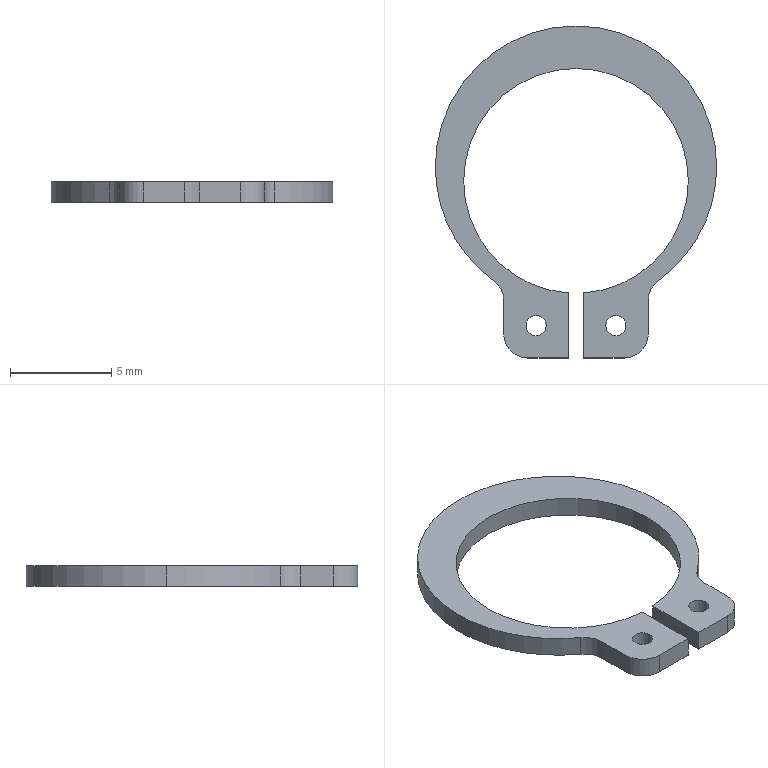Part | NX | features BREP 1 | 1 solid | 22 faces | box 13.9 x 16.4 x 1 mm | volume 70.676 mm3 | cylinder 14 | plane 8 | commonest cylinder face diameters 1 x4 2.38 x4 11.1 x3 13.9 x3
STEP:
#1=CARTESIAN_POINT('',(-2.47,-7.15,0.5));
#2=VERTEX_POINT('',#1);
#3=CARTESIAN_POINT('',(-1.47,-7.15,0.5));
#4=VERTEX_POINT('',#3);
#5=CARTESIAN_POINT('',(-1.97,-7.15,0.5));
#6=DIRECTION('',(0.,0.,1.));
#7=DIRECTION('',(1.,0.,0.));
#8=AXIS2_PLACEMENT_3D('',#5,#6,#7);
#9=CIRCLE('',#8,0.5);
#10=EDGE_CURVE('',#2,#4,#9,.T.);
#11=ORIENTED_EDGE('',*,*,#10,.T.);
#12=CARTESIAN_POINT('',(-1.47,-7.15,-0.5));
#13=VERTEX_POINT('',#12);
#14=CARTESIAN_POINT('',(-1.47,-7.15,0.5));
#15=DIRECTION('',(0.,0.,-1.));
#16=VECTOR('',#15,1000.);
#17=LINE('',#14,#16);
#18=EDGE_CURVE('',#13,#4,#17,.F.);
#19=ORIENTED_EDGE('',*,*,#18,.F.);
#20=CARTESIAN_POINT('',(-2.47,-7.15,-0.5));
#21=VERTEX_POINT('',#20);
#22=CARTESIAN_POINT('',(-1.97,-7.15,-0.5));
#23=DIRECTION('',(0.,0.,1.));
#24=DIRECTION('',(1.,0.,0.));
#25=AXIS2_PLACEMENT_3D('',#22,#23,#24);
#26=CIRCLE('',#25,0.5);
#27=EDGE_CURVE('',#21,#13,#26,.T.);
#28=ORIENTED_EDGE('',*,*,#27,.F.);
#29=CARTESIAN_POINT('',(-2.47,-7.15,0.5));
#30=DIRECTION('',(0.,0.,-1.));
#31=VECTOR('',#30,1000.);
#32=LINE('',#29,#31);
#33=EDGE_CURVE('',#21,#2,#32,.F.);
#34=ORIENTED_EDGE('',*,*,#33,.T.);
#35=EDGE_LOOP('',(#11,#19,#28,#34));
#36=FACE_BOUND('',#35,.T.);
#37=CARTESIAN_POINT('',(-1.97,-7.15,0.5));
#38=DIRECTION('',(0.,0.,-1.));
#39=DIRECTION('',(1.,0.,0.));
#40=AXIS2_PLACEMENT_3D('',#37,#38,#39);
#41=CYLINDRICAL_SURFACE('',#40,0.5);
#42=ADVANCED_FACE('',(#36),#41,.F.);
#43=CARTESIAN_POINT('',(1.47,-7.15,0.5));
#44=VERTEX_POINT('',#43);
#45=CARTESIAN_POINT('',(2.47,-7.15,0.5));
#46=VERTEX_POINT('',#45);
#47=CARTESIAN_POINT('',(1.97,-7.15,0.5));
#48=DIRECTION('',(0.,0.,1.));
#49=DIRECTION('',(1.,0.,0.));
#50=AXIS2_PLACEMENT_3D('',#47,#48,#49);
#51=CIRCLE('',#50,0.5);
#52=EDGE_CURVE('',#44,#46,#51,.T.);
#53=ORIENTED_EDGE('',*,*,#52,.T.);
#54=CARTESIAN_POINT('',(2.47,-7.15,-0.5));
#55=VERTEX_POINT('',#54);
#56=CARTESIAN_POINT('',(2.47,-7.15,0.5));
#57=DIRECTION('',(0.,0.,-1.));
#58=VECTOR('',#57,1000.);
#59=LINE('',#56,#58);
#60=EDGE_CURVE('',#55,#46,#59,.F.);
#61=ORIENTED_EDGE('',*,*,#60,.F.);
#62=CARTESIAN_POINT('',(1.47,-7.15,-0.5));
#63=VERTEX_POINT('',#62);
#64=CARTESIAN_POINT('',(1.97,-7.15,-0.5));
#65=DIRECTION('',(0.,0.,1.));
#66=DIRECTION('',(1.,0.,0.));
#67=AXIS2_PLACEMENT_3D('',#64,#65,#66);
#68=CIRCLE('',#67,0.5);
#69=EDGE_CURVE('',#63,#55,#68,.T.);
#70=ORIENTED_EDGE('',*,*,#69,.F.);
#71=CARTESIAN_POINT('',(1.47,-7.15,0.5));
#72=DIRECTION('',(0.,0.,-1.));
#73=VECTOR('',#72,1000.);
#74=LINE('',#71,#73);
#75=EDGE_CURVE('',#63,#44,#74,.F.);
#76=ORIENTED_EDGE('',*,*,#75,.T.);
#77=EDGE_LOOP('',(#53,#61,#70,#76));
#78=FACE_BOUND('',#77,.T.);
#79=CARTESIAN_POINT('',(1.97,-7.15,0.5));
#80=DIRECTION('',(0.,0.,-1.));
#81=DIRECTION('',(1.,0.,0.));
#82=AXIS2_PLACEMENT_3D('',#79,#80,#81);
#83=CYLINDRICAL_SURFACE('',#82,0.5);
#84=ADVANCED_FACE('',(#78),#83,.F.);
#85=CARTESIAN_POINT('',(5.55,0.,0.5));
#86=VERTEX_POINT('',#85);
#87=CARTESIAN_POINT('',(0.37,-5.538,0.5));
#88=VERTEX_POINT('',#87);
#89=CARTESIAN_POINT('',(0.,0.,0.5));
#90=DIRECTION('',(0.,0.,-1.));
#91=DIRECTION('',(-1.,0.,0.));
#92=AXIS2_PLACEMENT_3D('',#89,#90,#91);
#93=CIRCLE('',#92,5.55);
#94=EDGE_CURVE('',#86,#88,#93,.T.);
#95=ORIENTED_EDGE('',*,*,#94,.F.);
#96=CARTESIAN_POINT('',(5.55,0.,-0.5));
#97=VERTEX_POINT('',#96);
#98=CARTESIAN_POINT('',(5.55,0.,0.5));
#99=DIRECTION('',(0.,0.,-1.));
#100=VECTOR('',#99,1000.);
#101=LINE('',#98,#100);
#102=EDGE_CURVE('',#86,#97,#101,.T.);
#103=ORIENTED_EDGE('',*,*,#102,.T.);
#104=CARTESIAN_POINT('',(0.37,-5.538,-0.5));
#105=VERTEX_POINT('',#104);
#106=CARTESIAN_POINT('',(0.,0.,-0.5));
#107=DIRECTION('',(0.,0.,-1.));
#108=DIRECTION('',(-1.,0.,0.));
#109=AXIS2_PLACEMENT_3D('',#106,#107,#108);
#110=CIRCLE('',#109,5.55);
#111=EDGE_CURVE('',#97,#105,#110,.T.);
#112=ORIENTED_EDGE('',*,*,#111,.T.);
#113=CARTESIAN_POINT('',(0.37,-5.538,0.5));
#114=DIRECTION('',(0.,0.,-1.));
#115=VECTOR('',#114,1000.);
#116=LINE('',#113,#115);
#117=EDGE_CURVE('',#88,#105,#116,.T.);
#118=ORIENTED_EDGE('',*,*,#117,.F.);
#119=EDGE_LOOP('',(#95,#103,#112,#118));
#120=FACE_BOUND('',#119,.T.);
#121=CARTESIAN_POINT('',(0.,0.,0.5));
#122=DIRECTION('',(0.,0.,-1.));
#123=DIRECTION('',(1.,0.,0.));
#124=AXIS2_PLACEMENT_3D('',#121,#122,#123);
#125=CYLINDRICAL_SURFACE('',#124,5.55);
#126=ADVANCED_FACE('',(#120),#125,.F.);
#127=ORIENTED_EDGE('',*,*,#102,.F.);
#128=CARTESIAN_POINT('',(-5.55,0.,0.5));
#129=VERTEX_POINT('',#128);
#130=CARTESIAN_POINT('',(0.,0.,0.5));
#131=DIRECTION('',(0.,0.,-1.));
#132=DIRECTION('',(-1.,0.,0.));
#133=AXIS2_PLACEMENT_3D('',#130,#131,#132);
#134=CIRCLE('',#133,5.55);
#135=EDGE_CURVE('',#129,#86,#134,.T.);
#136=ORIENTED_EDGE('',*,*,#135,.F.);
#137=CARTESIAN_POINT('',(-5.55,0.,-0.5));
#138=VERTEX_POINT('',#137);
#139=CARTESIAN_POINT('',(-5.55,0.,0.5));
#140=DIRECTION('',(0.,0.,-1.));
#141=VECTOR('',#140,1000.);
#142=LINE('',#139,#141);
#143=EDGE_CURVE('',#129,#138,#142,.T.);
#144=ORIENTED_EDGE('',*,*,#143,.T.);
#145=CARTESIAN_POINT('',(0.,0.,-0.5));
#146=DIRECTION('',(0.,0.,-1.));
#147=DIRECTION('',(-1.,0.,0.));
#148=AXIS2_PLACEMENT_3D('',#145,#146,#147);
#149=CIRCLE('',#148,5.55);
#150=EDGE_CURVE('',#138,#97,#149,.T.);
#151=ORIENTED_EDGE('',*,*,#150,.T.);
#152=EDGE_LOOP('',(#127,#136,#144,#151));
#153=FACE_BOUND('',#152,.T.);
#154=CARTESIAN_POINT('',(0.,0.,0.5));
#155=DIRECTION('',(0.,0.,-1.));
#156=DIRECTION('',(1.,0.,0.));
#157=AXIS2_PLACEMENT_3D('',#154,#155,#156);
#158=CYLINDRICAL_SURFACE('',#157,5.55);
#159=ADVANCED_FACE('',(#153),#158,.F.);
#160=CARTESIAN_POINT('',(6.95,0.7,0.5));
#161=VERTEX_POINT('',#160);
#162=CARTESIAN_POINT('',(-6.95,0.7,0.5));
#163=VERTEX_POINT('',#162);
#164=CARTESIAN_POINT('',(0.,0.7,0.5));
#165=DIRECTION('',(0.,0.,1.));
#166=DIRECTION('',(1.,0.,0.));
#167=AXIS2_PLACEMENT_3D('',#164,#165,#166);
#168=CIRCLE('',#167,6.95);
#169=EDGE_CURVE('',#161,#163,#168,.T.);
#170=ORIENTED_EDGE('',*,*,#169,.F.);
#171=CARTESIAN_POINT('',(6.95,0.7,-0.5));
#172=VERTEX_POINT('',#171);
#173=CARTESIAN_POINT('',(6.95,0.7,0.5));
#174=DIRECTION('',(0.,0.,-1.));
#175=VECTOR('',#174,1000.);
#176=LINE('',#173,#175);
#177=EDGE_CURVE('',#161,#172,#176,.T.);
#178=ORIENTED_EDGE('',*,*,#177,.T.);
#179=CARTESIAN_POINT('',(-6.95,0.7,-0.5));
#180=VERTEX_POINT('',#179);
#181=CARTESIAN_POINT('',(0.,0.7,-0.5));
#182=DIRECTION('',(0.,0.,1.));
#183=DIRECTION('',(1.,0.,0.));
#184=AXIS2_PLACEMENT_3D('',#181,#182,#183);
#185=CIRCLE('',#184,6.95);
#186=EDGE_CURVE('',#172,#180,#185,.T.);
#187=ORIENTED_EDGE('',*,*,#186,.T.);
#188=CARTESIAN_POINT('',(-6.95,0.7,0.5));
#189=DIRECTION('',(0.,0.,-1.));
#190=VECTOR('',#189,1000.);
#191=LINE('',#188,#190);
#192=EDGE_CURVE('',#163,#180,#191,.T.);
#193=ORIENTED_EDGE('',*,*,#192,.F.);
#194=EDGE_LOOP('',(#170,#178,#187,#193));
#195=FACE_BOUND('',#194,.T.);
#196=CARTESIAN_POINT('',(0.,0.7,0.5));
#197=DIRECTION('',(0.,0.,-1.));
#198=DIRECTION('',(1.,0.,0.));
#199=AXIS2_PLACEMENT_3D('',#196,#197,#198);
#200=CYLINDRICAL_SURFACE('',#199,6.95);
#201=ADVANCED_FACE('',(#195),#200,.T.);
#202=CARTESIAN_POINT('',(-4.064,-4.938,0.5));
#203=VERTEX_POINT('',#202);
#204=CARTESIAN_POINT('',(0.,0.7,0.5));
#205=DIRECTION('',(0.,0.,1.));
#206=DIRECTION('',(1.,0.,0.));
#207=AXIS2_PLACEMENT_3D('',#204,#205,#206);
#208=CIRCLE('',#207,6.95);
#209=EDGE_CURVE('',#163,#203,#208,.T.);
#210=ORIENTED_EDGE('',*,*,#209,.F.);
#211=ORIENTED_EDGE('',*,*,#192,.T.);
#212=CARTESIAN_POINT('',(-4.064,-4.938,-0.5));
#213=VERTEX_POINT('',#212);
#214=CARTESIAN_POINT('',(0.,0.7,-0.5));
#215=DIRECTION('',(0.,0.,1.));
#216=DIRECTION('',(1.,0.,0.));
#217=AXIS2_PLACEMENT_3D('',#214,#215,#216);
#218=CIRCLE('',#217,6.95);
#219=EDGE_CURVE('',#180,#213,#218,.T.);
#220=ORIENTED_EDGE('',*,*,#219,.T.);
#221=CARTESIAN_POINT('',(-4.064,-4.938,0.5));
#222=DIRECTION('',(0.,0.,-1.));
#223=VECTOR('',#222,1000.);
#224=LINE('',#221,#223);
#225=EDGE_CURVE('',#203,#213,#224,.T.);
#226=ORIENTED_EDGE('',*,*,#225,.F.);
#227=EDGE_LOOP('',(#210,#211,#220,#226));
#228=FACE_BOUND('',#227,.T.);
#229=CARTESIAN_POINT('',(0.,0.7,0.5));
#230=DIRECTION('',(0.,0.,-1.));
#231=DIRECTION('',(1.,0.,0.));
#232=AXIS2_PLACEMENT_3D('',#229,#230,#231);
#233=CYLINDRICAL_SURFACE('',#232,6.95);
#234=ADVANCED_FACE('',(#228),#233,.T.);
#235=CARTESIAN_POINT('',(3.57,-5.903,0.5));
#236=VERTEX_POINT('',#235);
#237=CARTESIAN_POINT('',(4.064,-4.938,0.5));
#238=VERTEX_POINT('',#237);
#239=CARTESIAN_POINT('',(4.76,-5.903,0.5));
#240=DIRECTION('',(0.,0.,-1.));
#241=DIRECTION('',(-1.,0.,0.));
#242=AXIS2_PLACEMENT_3D('',#239,#240,#241);
#243=CIRCLE('',#242,1.19);
#244=EDGE_CURVE('',#236,#238,#243,.T.);
#245=ORIENTED_EDGE('',*,*,#244,.T.);
#246=CARTESIAN_POINT('',(0.,0.7,0.5));
#247=DIRECTION('',(0.,0.,1.));
#248=DIRECTION('',(1.,0.,0.));
#249=AXIS2_PLACEMENT_3D('',#246,#247,#248);
#250=CIRCLE('',#249,6.95);
#251=EDGE_CURVE('',#238,#161,#250,.T.);
#252=ORIENTED_EDGE('',*,*,#251,.T.);
#253=ORIENTED_EDGE('',*,*,#169,.T.);
#254=ORIENTED_EDGE('',*,*,#209,.T.);
#255=CARTESIAN_POINT('',(-3.57,-5.903,0.5));
#256=VERTEX_POINT('',#255);
#257=CARTESIAN_POINT('',(-4.76,-5.903,0.5));
#258=DIRECTION('',(0.,0.,-1.));
#259=DIRECTION('',(-1.,0.,0.));
#260=AXIS2_PLACEMENT_3D('',#257,#258,#259);
#261=CIRCLE('',#260,1.19);
#262=EDGE_CURVE('',#203,#256,#261,.T.);
#263=ORIENTED_EDGE('',*,*,#262,.T.);
#264=CARTESIAN_POINT('',(-3.57,-7.56,0.5));
#265=VERTEX_POINT('',#264);
#266=CARTESIAN_POINT('',(-3.57,-5.903,0.5));
#267=DIRECTION('',(0.,-1.,0.));
#268=VECTOR('',#267,1000.);
#269=LINE('',#266,#268);
#270=EDGE_CURVE('',#256,#265,#269,.T.);
#271=ORIENTED_EDGE('',*,*,#270,.T.);
#272=CARTESIAN_POINT('',(-2.38,-8.75,0.5));
#273=VERTEX_POINT('',#272);
#274=CARTESIAN_POINT('',(-2.38,-7.56,0.5));
#275=DIRECTION('',(0.,0.,1.));
#276=DIRECTION('',(1.,0.,0.));
#277=AXIS2_PLACEMENT_3D('',#274,#275,#276);
#278=CIRCLE('',#277,1.19);
#279=EDGE_CURVE('',#265,#273,#278,.T.);
#280=ORIENTED_EDGE('',*,*,#279,.T.);
#281=CARTESIAN_POINT('',(-0.37,-8.75,0.5));
#282=VERTEX_POINT('',#281);
#283=CARTESIAN_POINT('',(-2.38,-8.75,0.5));
#284=DIRECTION('',(1.,0.,0.));
#285=VECTOR('',#284,1000.);
#286=LINE('',#283,#285);
#287=EDGE_CURVE('',#273,#282,#286,.T.);
#288=ORIENTED_EDGE('',*,*,#287,.T.);
#289=CARTESIAN_POINT('',(-0.37,-5.538,0.5));
#290=VERTEX_POINT('',#289);
#291=CARTESIAN_POINT('',(-0.37,-8.75,0.5));
#292=DIRECTION('',(0.,1.,0.));
#293=VECTOR('',#292,1000.);
#294=LINE('',#291,#293);
#295=EDGE_CURVE('',#282,#290,#294,.T.);
#296=ORIENTED_EDGE('',*,*,#295,.T.);
#297=CARTESIAN_POINT('',(0.,0.,0.5));
#298=DIRECTION('',(0.,0.,-1.));
#299=DIRECTION('',(-1.,0.,0.));
#300=AXIS2_PLACEMENT_3D('',#297,#298,#299);
#301=CIRCLE('',#300,5.55);
#302=EDGE_CURVE('',#290,#129,#301,.T.);
#303=ORIENTED_EDGE('',*,*,#302,.T.);
#304=ORIENTED_EDGE('',*,*,#135,.T.);
#305=ORIENTED_EDGE('',*,*,#94,.T.);
#306=CARTESIAN_POINT('',(0.37,-8.75,0.5));
#307=VERTEX_POINT('',#306);
#308=CARTESIAN_POINT('',(0.37,-5.538,0.5));
#309=DIRECTION('',(0.,-1.,0.));
#310=VECTOR('',#309,1000.);
#311=LINE('',#308,#310);
#312=EDGE_CURVE('',#88,#307,#311,.T.);
#313=ORIENTED_EDGE('',*,*,#312,.T.);
#314=CARTESIAN_POINT('',(2.38,-8.75,0.5));
#315=VERTEX_POINT('',#314);
#316=CARTESIAN_POINT('',(0.37,-8.75,0.5));
#317=DIRECTION('',(1.,0.,0.));
#318=VECTOR('',#317,1000.);
#319=LINE('',#316,#318);
#320=EDGE_CURVE('',#307,#315,#319,.T.);
#321=ORIENTED_EDGE('',*,*,#320,.T.);
#322=CARTESIAN_POINT('',(3.57,-7.56,0.5));
#323=VERTEX_POINT('',#322);
#324=CARTESIAN_POINT('',(2.38,-7.56,0.5));
#325=DIRECTION('',(0.,0.,1.));
#326=DIRECTION('',(1.,0.,0.));
#327=AXIS2_PLACEMENT_3D('',#324,#325,#326);
#328=CIRCLE('',#327,1.19);
#329=EDGE_CURVE('',#315,#323,#328,.T.);
#330=ORIENTED_EDGE('',*,*,#329,.T.);
#331=CARTESIAN_POINT('',(3.57,-7.56,0.5));
#332=DIRECTION('',(0.,1.,0.));
#333=VECTOR('',#332,1000.);
#334=LINE('',#331,#333);
#335=EDGE_CURVE('',#323,#236,#334,.T.);
#336=ORIENTED_EDGE('',*,*,#335,.T.);
#337=EDGE_LOOP('',(#245,#252,#253,#254,#263,#271,#280,#288,#296,#303,#304,#305,#313,#321,#330,#336));
#338=FACE_BOUND('',#337,.T.);
#339=ORIENTED_EDGE('',*,*,#52,.F.);
#340=CARTESIAN_POINT('',(1.97,-7.15,0.5));
#341=DIRECTION('',(0.,0.,1.));
#342=DIRECTION('',(1.,0.,0.));
#343=AXIS2_PLACEMENT_3D('',#340,#341,#342);
#344=CIRCLE('',#343,0.5);
#345=EDGE_CURVE('',#46,#44,#344,.T.);
#346=ORIENTED_EDGE('',*,*,#345,.F.);
#347=EDGE_LOOP('',(#339,#346));
#348=FACE_BOUND('',#347,.T.);
#349=ORIENTED_EDGE('',*,*,#10,.F.);
#350=CARTESIAN_POINT('',(-1.97,-7.15,0.5));
#351=DIRECTION('',(0.,0.,1.));
#352=DIRECTION('',(1.,0.,0.));
#353=AXIS2_PLACEMENT_3D('',#350,#351,#352);
#354=CIRCLE('',#353,0.5);
#355=EDGE_CURVE('',#4,#2,#354,.T.);
#356=ORIENTED_EDGE('',*,*,#355,.F.);
#357=EDGE_LOOP('',(#349,#356));
#358=FACE_BOUND('',#357,.T.);
#359=CARTESIAN_POINT('',(4.76,-5.903,0.5));
#360=DIRECTION('',(0.,0.,-1.));
#361=DIRECTION('',(1.,0.,0.));
#362=AXIS2_PLACEMENT_3D('',#359,#360,#361);
#363=PLANE('',#362);
#364=ADVANCED_FACE('',(#338,#348,#358),#363,.F.);
#365=CARTESIAN_POINT('',(3.57,-5.903,-0.5));
#366=VERTEX_POINT('',#365);
#367=CARTESIAN_POINT('',(3.57,-5.903,0.5));
#368=DIRECTION('',(0.,0.,-1.));
#369=VECTOR('',#368,1000.);
#370=LINE('',#367,#369);
#371=EDGE_CURVE('',#236,#366,#370,.T.);
#372=ORIENTED_EDGE('',*,*,#371,.T.);
#373=CARTESIAN_POINT('',(4.064,-4.938,-0.5));
#374=VERTEX_POINT('',#373);
#375=CARTESIAN_POINT('',(4.76,-5.903,-0.5));
#376=DIRECTION('',(0.,0.,-1.));
#377=DIRECTION('',(-1.,0.,0.));
#378=AXIS2_PLACEMENT_3D('',#375,#376,#377);
#379=CIRCLE('',#378,1.19);
#380=EDGE_CURVE('',#366,#374,#379,.T.);
#381=ORIENTED_EDGE('',*,*,#380,.T.);
#382=CARTESIAN_POINT('',(4.064,-4.938,0.5));
#383=DIRECTION('',(0.,0.,-1.));
#384=VECTOR('',#383,1000.);
#385=LINE('',#382,#384);
#386=EDGE_CURVE('',#238,#374,#385,.T.);
#387=ORIENTED_EDGE('',*,*,#386,.F.);
#388=ORIENTED_EDGE('',*,*,#244,.F.);
#389=EDGE_LOOP('',(#372,#381,#387,#388));
#390=FACE_BOUND('',#389,.T.);
#391=CARTESIAN_POINT('',(4.76,-5.903,0.5));
#392=DIRECTION('',(0.,0.,-1.));
#393=DIRECTION('',(1.,0.,0.));
#394=AXIS2_PLACEMENT_3D('',#391,#392,#393);
#395=CYLINDRICAL_SURFACE('',#394,1.19);
#396=ADVANCED_FACE('',(#390),#395,.F.);
#397=ORIENTED_EDGE('',*,*,#177,.F.);
#398=ORIENTED_EDGE('',*,*,#251,.F.);
#399=ORIENTED_EDGE('',*,*,#386,.T.);
#400=CARTESIAN_POINT('',(0.,0.7,-0.5));
#401=DIRECTION('',(0.,0.,1.));
#402=DIRECTION('',(1.,0.,0.));
#403=AXIS2_PLACEMENT_3D('',#400,#401,#402);
#404=CIRCLE('',#403,6.95);
#405=EDGE_CURVE('',#374,#172,#404,.T.);
#406=ORIENTED_EDGE('',*,*,#405,.T.);
#407=EDGE_LOOP('',(#397,#398,#399,#406));
#408=FACE_BOUND('',#407,.T.);
#409=CARTESIAN_POINT('',(0.,0.7,0.5));
#410=DIRECTION('',(0.,0.,-1.));
#411=DIRECTION('',(1.,0.,0.));
#412=AXIS2_PLACEMENT_3D('',#409,#410,#411);
#413=CYLINDRICAL_SURFACE('',#412,6.95);
#414=ADVANCED_FACE('',(#408),#413,.T.);
#415=ORIENTED_EDGE('',*,*,#225,.T.);
#416=CARTESIAN_POINT('',(-3.57,-5.903,-0.5));
#417=VERTEX_POINT('',#416);
#418=CARTESIAN_POINT('',(-4.76,-5.903,-0.5));
#419=DIRECTION('',(0.,0.,-1.));
#420=DIRECTION('',(-1.,0.,0.));
#421=AXIS2_PLACEMENT_3D('',#418,#419,#420);
#422=CIRCLE('',#421,1.19);
#423=EDGE_CURVE('',#213,#417,#422,.T.);
#424=ORIENTED_EDGE('',*,*,#423,.T.);
#425=CARTESIAN_POINT('',(-3.57,-5.903,0.5));
#426=DIRECTION('',(0.,0.,-1.));
#427=VECTOR('',#426,1000.);
#428=LINE('',#425,#427);
#429=EDGE_CURVE('',#256,#417,#428,.T.);
#430=ORIENTED_EDGE('',*,*,#429,.F.);
#431=ORIENTED_EDGE('',*,*,#262,.F.);
#432=EDGE_LOOP('',(#415,#424,#430,#431));
#433=FACE_BOUND('',#432,.T.);
#434=CARTESIAN_POINT('',(-4.76,-5.903,0.5));
#435=DIRECTION('',(0.,0.,-1.));
#436=DIRECTION('',(1.,0.,0.));
#437=AXIS2_PLACEMENT_3D('',#434,#435,#436);
#438=CYLINDRICAL_SURFACE('',#437,1.19);
#439=ADVANCED_FACE('',(#433),#438,.F.);
#440=ORIENTED_EDGE('',*,*,#429,.T.);
#441=CARTESIAN_POINT('',(-3.57,-7.56,-0.5));
#442=VERTEX_POINT('',#441);
#443=CARTESIAN_POINT('',(-3.57,-5.903,-0.5));
#444=DIRECTION('',(0.,-1.,0.));
#445=VECTOR('',#444,1000.);
#446=LINE('',#443,#445);
#447=EDGE_CURVE('',#417,#442,#446,.T.);
#448=ORIENTED_EDGE('',*,*,#447,.T.);
#449=CARTESIAN_POINT('',(-3.57,-7.56,0.5));
#450=DIRECTION('',(0.,0.,-1.));
#451=VECTOR('',#450,1000.);
#452=LINE('',#449,#451);
#453=EDGE_CURVE('',#265,#442,#452,.T.);
#454=ORIENTED_EDGE('',*,*,#453,.F.);
#455=ORIENTED_EDGE('',*,*,#270,.F.);
#456=EDGE_LOOP('',(#440,#448,#454,#455));
#457=FACE_BOUND('',#456,.T.);
#458=CARTESIAN_POINT('',(-3.57,-5.903,0.5));
#459=DIRECTION('',(1.,0.,0.));
#460=DIRECTION('',(0.,0.,1.));
#461=AXIS2_PLACEMENT_3D('',#458,#459,#460);
#462=PLANE('',#461);
#463=ADVANCED_FACE('',(#457),#462,.F.);
#464=ORIENTED_EDGE('',*,*,#453,.T.);
#465=CARTESIAN_POINT('',(-2.38,-8.75,-0.5));
#466=VERTEX_POINT('',#465);
#467=CARTESIAN_POINT('',(-2.38,-7.56,-0.5));
#468=DIRECTION('',(0.,0.,1.));
#469=DIRECTION('',(1.,0.,0.));
#470=AXIS2_PLACEMENT_3D('',#467,#468,#469);
#471=CIRCLE('',#470,1.19);
#472=EDGE_CURVE('',#442,#466,#471,.T.);
#473=ORIENTED_EDGE('',*,*,#472,.T.);
#474=CARTESIAN_POINT('',(-2.38,-8.75,0.5));
#475=DIRECTION('',(0.,0.,-1.));
#476=VECTOR('',#475,1000.);
#477=LINE('',#474,#476);
#478=EDGE_CURVE('',#273,#466,#477,.T.);
#479=ORIENTED_EDGE('',*,*,#478,.F.);
#480=ORIENTED_EDGE('',*,*,#279,.F.);
#481=EDGE_LOOP('',(#464,#473,#479,#480));
#482=FACE_BOUND('',#481,.T.);
#483=CARTESIAN_POINT('',(-2.38,-7.56,0.5));
#484=DIRECTION('',(0.,0.,-1.));
#485=DIRECTION('',(1.,0.,0.));
#486=AXIS2_PLACEMENT_3D('',#483,#484,#485);
#487=CYLINDRICAL_SURFACE('',#486,1.19);
#488=ADVANCED_FACE('',(#482),#487,.T.);
#489=ORIENTED_EDGE('',*,*,#478,.T.);
#490=CARTESIAN_POINT('',(-0.37,-8.75,-0.5));
#491=VERTEX_POINT('',#490);
#492=CARTESIAN_POINT('',(-2.38,-8.75,-0.5));
#493=DIRECTION('',(1.,0.,0.));
#494=VECTOR('',#493,1000.);
#495=LINE('',#492,#494);
#496=EDGE_CURVE('',#466,#491,#495,.T.);
#497=ORIENTED_EDGE('',*,*,#496,.T.);
#498=CARTESIAN_POINT('',(-0.37,-8.75,0.5));
#499=DIRECTION('',(0.,0.,-1.));
#500=VECTOR('',#499,1000.);
#501=LINE('',#498,#500);
#502=EDGE_CURVE('',#282,#491,#501,.T.);
#503=ORIENTED_EDGE('',*,*,#502,.F.);
#504=ORIENTED_EDGE('',*,*,#287,.F.);
#505=EDGE_LOOP('',(#489,#497,#503,#504));
#506=FACE_BOUND('',#505,.T.);
#507=CARTESIAN_POINT('',(-2.38,-8.75,0.5));
#508=DIRECTION('',(0.,1.,0.));
#509=DIRECTION('',(0.,0.,-1.));
#510=AXIS2_PLACEMENT_3D('',#507,#508,#509);
#511=PLANE('',#510);
#512=ADVANCED_FACE('',(#506),#511,.F.);
#513=ORIENTED_EDGE('',*,*,#502,.T.);
#514=CARTESIAN_POINT('',(-0.37,-5.538,-0.5));
#515=VERTEX_POINT('',#514);
#516=CARTESIAN_POINT('',(-0.37,-8.75,-0.5));
#517=DIRECTION('',(0.,1.,0.));
#518=VECTOR('',#517,1000.);
#519=LINE('',#516,#518);
#520=EDGE_CURVE('',#491,#515,#519,.T.);
#521=ORIENTED_EDGE('',*,*,#520,.T.);
#522=CARTESIAN_POINT('',(-0.37,-5.538,0.5));
#523=DIRECTION('',(0.,0.,-1.));
#524=VECTOR('',#523,1000.);
#525=LINE('',#522,#524);
#526=EDGE_CURVE('',#290,#515,#525,.T.);
#527=ORIENTED_EDGE('',*,*,#526,.F.);
#528=ORIENTED_EDGE('',*,*,#295,.F.);
#529=EDGE_LOOP('',(#513,#521,#527,#528));
#530=FACE_BOUND('',#529,.T.);
#531=CARTESIAN_POINT('',(-0.37,-8.75,0.5));
#532=DIRECTION('',(-1.,0.,0.));
#533=DIRECTION('',(0.,0.,-1.));
#534=AXIS2_PLACEMENT_3D('',#531,#532,#533);
#535=PLANE('',#534);
#536=ADVANCED_FACE('',(#530),#535,.F.);
#537=ORIENTED_EDGE('',*,*,#143,.F.);
#538=ORIENTED_EDGE('',*,*,#302,.F.);
#539=ORIENTED_EDGE('',*,*,#526,.T.);
#540=CARTESIAN_POINT('',(0.,0.,-0.5));
#541=DIRECTION('',(0.,0.,-1.));
#542=DIRECTION('',(-1.,0.,0.));
#543=AXIS2_PLACEMENT_3D('',#540,#541,#542);
#544=CIRCLE('',#543,5.55);
#545=EDGE_CURVE('',#515,#138,#544,.T.);
#546=ORIENTED_EDGE('',*,*,#545,.T.);
#547=EDGE_LOOP('',(#537,#538,#539,#546));
#548=FACE_BOUND('',#547,.T.);
#549=CARTESIAN_POINT('',(0.,0.,0.5));
#550=DIRECTION('',(0.,0.,-1.));
#551=DIRECTION('',(1.,0.,0.));
#552=AXIS2_PLACEMENT_3D('',#549,#550,#551);
#553=CYLINDRICAL_SURFACE('',#552,5.55);
#554=ADVANCED_FACE('',(#548),#553,.F.);
#555=ORIENTED_EDGE('',*,*,#117,.T.);
#556=CARTESIAN_POINT('',(0.37,-8.75,-0.5));
#557=VERTEX_POINT('',#556);
#558=CARTESIAN_POINT('',(0.37,-5.538,-0.5));
#559=DIRECTION('',(0.,-1.,0.));
#560=VECTOR('',#559,1000.);
#561=LINE('',#558,#560);
#562=EDGE_CURVE('',#105,#557,#561,.T.);
#563=ORIENTED_EDGE('',*,*,#562,.T.);
#564=CARTESIAN_POINT('',(0.37,-8.75,0.5));
#565=DIRECTION('',(0.,0.,-1.));
#566=VECTOR('',#565,1000.);
#567=LINE('',#564,#566);
#568=EDGE_CURVE('',#307,#557,#567,.T.);
#569=ORIENTED_EDGE('',*,*,#568,.F.);
#570=ORIENTED_EDGE('',*,*,#312,.F.);
#571=EDGE_LOOP('',(#555,#563,#569,#570));
#572=FACE_BOUND('',#571,.T.);
#573=CARTESIAN_POINT('',(0.37,-5.538,0.5));
#574=DIRECTION('',(1.,0.,0.));
#575=DIRECTION('',(0.,0.,1.));
#576=AXIS2_PLACEMENT_3D('',#573,#574,#575);
#577=PLANE('',#576);
#578=ADVANCED_FACE('',(#572),#577,.F.);
#579=ORIENTED_EDGE('',*,*,#568,.T.);
#580=CARTESIAN_POINT('',(2.38,-8.75,-0.5));
#581=VERTEX_POINT('',#580);
#582=CARTESIAN_POINT('',(0.37,-8.75,-0.5));
#583=DIRECTION('',(1.,0.,0.));
#584=VECTOR('',#583,1000.);
#585=LINE('',#582,#584);
#586=EDGE_CURVE('',#557,#581,#585,.T.);
#587=ORIENTED_EDGE('',*,*,#586,.T.);
#588=CARTESIAN_POINT('',(2.38,-8.75,0.5));
#589=DIRECTION('',(0.,0.,-1.));
#590=VECTOR('',#589,1000.);
#591=LINE('',#588,#590);
#592=EDGE_CURVE('',#315,#581,#591,.T.);
#593=ORIENTED_EDGE('',*,*,#592,.F.);
#594=ORIENTED_EDGE('',*,*,#320,.F.);
#595=EDGE_LOOP('',(#579,#587,#593,#594));
#596=FACE_BOUND('',#595,.T.);
#597=CARTESIAN_POINT('',(0.37,-8.75,0.5));
#598=DIRECTION('',(0.,1.,0.));
#599=DIRECTION('',(0.,0.,-1.));
#600=AXIS2_PLACEMENT_3D('',#597,#598,#599);
#601=PLANE('',#600);
#602=ADVANCED_FACE('',(#596),#601,.F.);
#603=ORIENTED_EDGE('',*,*,#592,.T.);
#604=CARTESIAN_POINT('',(3.57,-7.56,-0.5));
#605=VERTEX_POINT('',#604);
#606=CARTESIAN_POINT('',(2.38,-7.56,-0.5));
#607=DIRECTION('',(0.,0.,1.));
#608=DIRECTION('',(1.,0.,0.));
#609=AXIS2_PLACEMENT_3D('',#606,#607,#608);
#610=CIRCLE('',#609,1.19);
#611=EDGE_CURVE('',#581,#605,#610,.T.);
#612=ORIENTED_EDGE('',*,*,#611,.T.);
#613=CARTESIAN_POINT('',(3.57,-7.56,0.5));
#614=DIRECTION('',(0.,0.,-1.));
#615=VECTOR('',#614,1000.);
#616=LINE('',#613,#615);
#617=EDGE_CURVE('',#323,#605,#616,.T.);
#618=ORIENTED_EDGE('',*,*,#617,.F.);
#619=ORIENTED_EDGE('',*,*,#329,.F.);
#620=EDGE_LOOP('',(#603,#612,#618,#619));
#621=FACE_BOUND('',#620,.T.);
#622=CARTESIAN_POINT('',(2.38,-7.56,0.5));
#623=DIRECTION('',(0.,0.,-1.));
#624=DIRECTION('',(1.,0.,0.));
#625=AXIS2_PLACEMENT_3D('',#622,#623,#624);
#626=CYLINDRICAL_SURFACE('',#625,1.19);
#627=ADVANCED_FACE('',(#621),#626,.T.);
#628=ORIENTED_EDGE('',*,*,#617,.T.);
#629=CARTESIAN_POINT('',(3.57,-7.56,-0.5));
#630=DIRECTION('',(0.,1.,0.));
#631=VECTOR('',#630,1000.);
#632=LINE('',#629,#631);
#633=EDGE_CURVE('',#605,#366,#632,.T.);
#634=ORIENTED_EDGE('',*,*,#633,.T.);
#635=ORIENTED_EDGE('',*,*,#371,.F.);
#636=ORIENTED_EDGE('',*,*,#335,.F.);
#637=EDGE_LOOP('',(#628,#634,#635,#636));
#638=FACE_BOUND('',#637,.T.);
#639=CARTESIAN_POINT('',(3.57,-7.56,0.5));
#640=DIRECTION('',(-1.,0.,0.));
#641=DIRECTION('',(0.,0.,-1.));
#642=AXIS2_PLACEMENT_3D('',#639,#640,#641);
#643=PLANE('',#642);
#644=ADVANCED_FACE('',(#638),#643,.F.);
#645=ORIENTED_EDGE('',*,*,#60,.T.);
#646=ORIENTED_EDGE('',*,*,#345,.T.);
#647=ORIENTED_EDGE('',*,*,#75,.F.);
#648=CARTESIAN_POINT('',(1.97,-7.15,-0.5));
#649=DIRECTION('',(0.,0.,1.));
#650=DIRECTION('',(1.,0.,0.));
#651=AXIS2_PLACEMENT_3D('',#648,#649,#650);
#652=CIRCLE('',#651,0.5);
#653=EDGE_CURVE('',#55,#63,#652,.T.);
#654=ORIENTED_EDGE('',*,*,#653,.F.);
#655=EDGE_LOOP('',(#645,#646,#647,#654));
#656=FACE_BOUND('',#655,.T.);
#657=CARTESIAN_POINT('',(1.97,-7.15,0.5));
#658=DIRECTION('',(0.,0.,-1.));
#659=DIRECTION('',(1.,0.,0.));
#660=AXIS2_PLACEMENT_3D('',#657,#658,#659);
#661=CYLINDRICAL_SURFACE('',#660,0.5);
#662=ADVANCED_FACE('',(#656),#661,.F.);
#663=ORIENTED_EDGE('',*,*,#18,.T.);
#664=ORIENTED_EDGE('',*,*,#355,.T.);
#665=ORIENTED_EDGE('',*,*,#33,.F.);
#666=CARTESIAN_POINT('',(-1.97,-7.15,-0.5));
#667=DIRECTION('',(0.,0.,1.));
#668=DIRECTION('',(1.,0.,0.));
#669=AXIS2_PLACEMENT_3D('',#666,#667,#668);
#670=CIRCLE('',#669,0.5);
#671=EDGE_CURVE('',#13,#21,#670,.T.);
#672=ORIENTED_EDGE('',*,*,#671,.F.);
#673=EDGE_LOOP('',(#663,#664,#665,#672));
#674=FACE_BOUND('',#673,.T.);
#675=CARTESIAN_POINT('',(-1.97,-7.15,0.5));
#676=DIRECTION('',(0.,0.,-1.));
#677=DIRECTION('',(1.,0.,0.));
#678=AXIS2_PLACEMENT_3D('',#675,#676,#677);
#679=CYLINDRICAL_SURFACE('',#678,0.5);
#680=ADVANCED_FACE('',(#674),#679,.F.);
#681=ORIENTED_EDGE('',*,*,#27,.T.);
#682=ORIENTED_EDGE('',*,*,#671,.T.);
#683=EDGE_LOOP('',(#681,#682));
#684=FACE_BOUND('',#683,.T.);
#685=ORIENTED_EDGE('',*,*,#69,.T.);
#686=ORIENTED_EDGE('',*,*,#653,.T.);
#687=EDGE_LOOP('',(#685,#686));
#688=FACE_BOUND('',#687,.T.);
#689=ORIENTED_EDGE('',*,*,#380,.F.);
#690=ORIENTED_EDGE('',*,*,#633,.F.);
#691=ORIENTED_EDGE('',*,*,#611,.F.);
#692=ORIENTED_EDGE('',*,*,#586,.F.);
#693=ORIENTED_EDGE('',*,*,#562,.F.);
#694=ORIENTED_EDGE('',*,*,#111,.F.);
#695=ORIENTED_EDGE('',*,*,#150,.F.);
#696=ORIENTED_EDGE('',*,*,#545,.F.);
#697=ORIENTED_EDGE('',*,*,#520,.F.);
#698=ORIENTED_EDGE('',*,*,#496,.F.);
#699=ORIENTED_EDGE('',*,*,#472,.F.);
#700=ORIENTED_EDGE('',*,*,#447,.F.);
#701=ORIENTED_EDGE('',*,*,#423,.F.);
#702=ORIENTED_EDGE('',*,*,#219,.F.);
#703=ORIENTED_EDGE('',*,*,#186,.F.);
#704=ORIENTED_EDGE('',*,*,#405,.F.);
#705=EDGE_LOOP('',(#689,#690,#691,#692,#693,#694,#695,#696,#697,#698,#699,#700,#701,#702,#703,#704));
#706=FACE_BOUND('',#705,.T.);
#707=CARTESIAN_POINT('',(4.76,-5.903,-0.5));
#708=DIRECTION('',(0.,0.,-1.));
#709=DIRECTION('',(1.,0.,0.));
#710=AXIS2_PLACEMENT_3D('',#707,#708,#709);
#711=PLANE('',#710);
#712=ADVANCED_FACE('',(#684,#688,#706),#711,.T.);
#713=CLOSED_SHELL('',(#42,#84,#126,#159,#201,#234,#364,#396,#414,#439,#463,#488,#512,#536,#554,#578,#602,#627,#644,#662,#680,#712));
#714=MANIFOLD_SOLID_BREP('',#713);
#715=(LENGTH_UNIT()NAMED_UNIT(*)SI_UNIT(.MILLI.,.METRE.));
#716=UNCERTAINTY_MEASURE_WITH_UNIT(LENGTH_MEASURE(0.00001),#715,'','');
#717=(NAMED_UNIT(*)PLANE_ANGLE_UNIT()SI_UNIT($,.RADIAN.));
#718=(NAMED_UNIT(*)SI_UNIT($,.STERADIAN.)SOLID_ANGLE_UNIT());
#719=(GEOMETRIC_REPRESENTATION_CONTEXT(3)GLOBAL_UNCERTAINTY_ASSIGNED_CONTEXT((#716))GLOBAL_UNIT_ASSIGNED_CONTEXT((#715,#717,#718))REPRESENTATION_CONTEXT('',''));
#720=ADVANCED_BREP_SHAPE_REPRESENTATION('',(#714),#719);